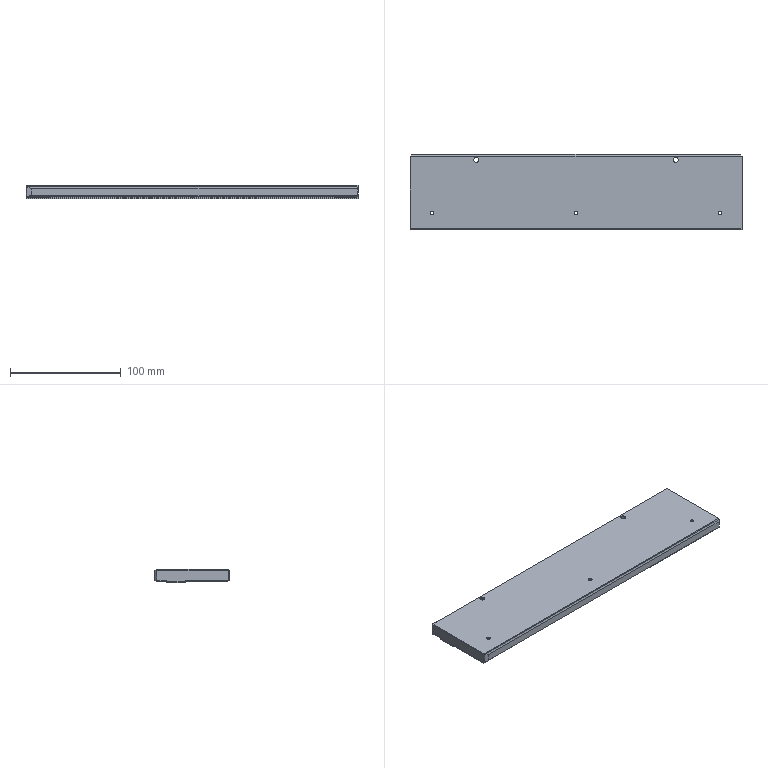CAM job | NX | 3-axis milling, drilling | part box 300 x 68 x 12 mm | stock box 305 x 73 x 15 mm
Tools:
number,name,description,diameter,corner_radius,flute_length,length,flutes
6,D6,平底铣刀-粗,6.0,0.0,25.0,75.0,2
9,D10,平底铣刀-粗,10.0,0.0,35.0,75.0,2
7,D6-J,平底铣刀-精,6.0,0.0,25.0,75.0,2
10,D10-J,平底铣刀-精,10.0,0.0,35.0,75.0,2
17,D6R0.5,圆鼻刀-粗,6.0,0.5,50.0,75.0,2
2,D6倒角刀,倒角刀,6.0,0.0,3.0,25.0,2
21,M4X0.7,丝锥,3.3,0.0,35.0,50.0,2
13,ZT3.3,钻头,3.3,0.0,35.0,50.0,2
11,ZT4.5,钻头,4.5,0.0,35.0,50.0,2
Operations:
program,operation,operation_type,tool,method,geometry_group,spindle_rpm,surface_speed,feed_per_tooth,feed_cut,feed_plunge,cut_length_mm,path_length_mm,cut_time_min,machine_time_min
D,顶面_COPY_COPY,FaceMilling,D10-J,侧刃精光-切深K-步距G,W-D,4500.0,1385.0,0.1667,1500.0,100.0,7823.056,8189.725,5.215,5.252
D,面铣自动飞面精光_COPY_COPY_COPY,FaceMilling,D10-J,侧刃精光-切深K-步距G,W-D,8000.0,251.327,0.0625,1000.0,100.0,3931.327,3987.327,3.931,3.937
D,底壁铣分层开粗-中_COPY_1,VolumeBased25DMillingOperation,D6,分层开粗-切深K-步距G,W-D,8000.0,150.792,0.1875,3000.0,100.0,12108.7,12867.011,4.036,4.112
D,打点-深0.8,Operation,D6倒角刀,NONE,W-D,8000.0,150.796,0.0312,500.0,90.0,9.0,413.39,0.018,0.0584
D,通孔-M4螺纹底孔,Operation,ZT3.3,NONE,W-D,3000.0,30.536,0.05,300.0,90.0,45.0,414.408,0.15,0.1869
D,通孔-5-6,Operation,ZT4.5,NONE,W-D,3000.0,42.411,0.025,150.0,90.0,26.304,296.01,0.1754,0.2023
D,钻倒角_3,Operation,D6倒角刀,METHOD,W-D,8000.0,150.796,0.0312,500.0,0.0,15.513,359.495,0.031,0.0654
D,铣倒角_1,PlanarMilling,D6倒角刀,METHOD,W-D,8000.0,150.796,0.0312,500.0,100.0,34.706,341.509,0.0694,0.1001
D,平面去毛刺6X45L_COPY_2,SurfaceContour,D6倒角刀,爬面_倒角-切深0-步距G,W-D,6500.0,122.519,0.1154,1500.0,100.0,823.26,2832.396,0.5488,0.7498
D,底壁铣倒角_COPY_2,VolumeBased25DMillingOperation,D6倒角刀,爬面_倒角-切深0-步距G,W-D,6500.0,122.519,0.1154,1500.0,100.0,620.85,816.257,0.4139,0.4334
D,通孔-攻牙M4,Operation,M4X0.7,METHOD,W-D,600.0,6.22,0.0006,0.7,90.0,3.0,330.408,4.286,4.319
D,底壁铣精光底面-中_COPY_1,VolumeBased25DMillingOperation,D6-J,精光步距切深关,W-D,8000.0,150.792,0.0625,1000.0,100.0,5468.189,5566.134,5.468,5.478
D,底壁铣精光侧面-中-选底面_COPY_1,VolumeBased25DMillingOperation,D6-J,侧刃精光-切深K-步距G,W-D,8000.0,150.792,0.0625,1000.0,100.0,624.335,680.533,0.6243,0.63
C,顶面_COPY,FaceMilling,D10-J,侧刃精光-切深K-步距G,W-C,4500.0,1385.0,0.1667,1500.0,100.0,7823.056,8205.425,5.215,5.254
C,面铣自动飞面精光_COPY_COPY,FaceMilling,D10-J,侧刃精光-切深K-步距G,W-C,8000.0,251.327,0.0625,1000.0,100.0,3931.327,3987.327,3.931,3.937
C,钻倒角_1,Operation,D6倒角刀,METHOD,W-C,8000.0,150.796,0.0625,1000.0,0.0,14.763,355.595,0.0148,0.0488
C,钻倒角_2,Operation,D6倒角刀,METHOD,W-C,8000.0,150.796,0.0625,1000.0,0.0,11.1,265.225,0.0111,0.0365
C,平面去毛刺6X45L_COPY_1,SurfaceContour,D6倒角刀,爬面_倒角-切深0-步距G,W-C,6500.0,122.519,0.1154,1500.0,100.0,495.988,1032.929,0.3307,0.3844
C,底壁铣倒角_COPY_1,VolumeBased25DMillingOperation,D6倒角刀,爬面_倒角-切深0-步距G,W-C,6500.0,122.519,0.1154,1500.0,100.0,309.185,368.585,0.2061,0.2121
C,等高精光往复爬面_COPY,ZLevelMilling,D6R0.5,等高爬面-切深K-步距G,W-C,8000.0,150.796,0.2812,4500.0,100.0,7824.863,7849.114,1.739,1.741
B,面铣自动飞面开粗_COPY,FaceMilling,D10-J,分层开粗-切深K-步距G,W-B,8000.0,251.327,0.1875,3000.0,100.0,19466.227,20921.016,6.489,6.634
B,面铣自动飞面精光_COPY,FaceMilling,D10-J,侧刃精光-切深K-步距G,W-B,8000.0,251.327,0.0625,1000.0,100.0,3931.327,4027.327,3.931,3.941
B,底壁铣分层开粗-中_COPY,VolumeBased25DMillingOperation,D6,分层开粗-切深K-步距G,W-B,8000.0,150.792,0.1875,3000.0,100.0,11186.272,12524.911,3.729,3.863
B,底壁铣精光底面-中_COPY,VolumeBased25DMillingOperation,D6-J,精光步距切深关,W-B,8000.0,150.792,0.0625,1000.0,100.0,5454.738,5577.047,5.455,5.467
B,底壁铣精光侧面-中-选底面_COPY,VolumeBased25DMillingOperation,D6-J,侧刃精光-切深K-步距G,W-B,8000.0,150.792,0.0625,1000.0,100.0,624.335,683.533,0.6243,0.6303
B,平面去毛刺6X45L_COPY,SurfaceContour,D6倒角刀,爬面_倒角-切深0-步距G,W-B,6500.0,122.519,0.1154,1500.0,100.0,762.198,1708.943,0.5081,0.6028
B,底壁铣倒角_COPY,VolumeBased25DMillingOperation,D6倒角刀,爬面_倒角-切深0-步距G,W-B,6500.0,122.519,0.1154,1500.0,100.0,617.393,895.824,0.4116,0.4394
A,顶面,FaceMilling,D10-J,侧刃精光-切深K-步距G,W-A,4500.0,1385.0,0.1667,1500.0,100.0,3911.528,3967.528,2.608,2.613
A,外形粗_2,VolumeBased25DMillingOperation,D10,METHOD,W-A,8000.0,251.327,0.375,6000.0,80.0,13000.982,13071.482,2.167,2.174
A,C0.3封闭铣廓倒角6X45L_COPY,PlanarMilling,D6倒角刀,爬面_倒角-切深0-步距G,W-A,7000.0,131.0,0.1071,1500.0,100.0,750.163,806.163,0.5001,0.5057
A,外形半精_2,VolumeBased25DMillingOperation,D10-J,METHOD,W-A,9000.0,169.646,0.0667,1200.0,100.0,769.005,852.005,0.6408,0.6491